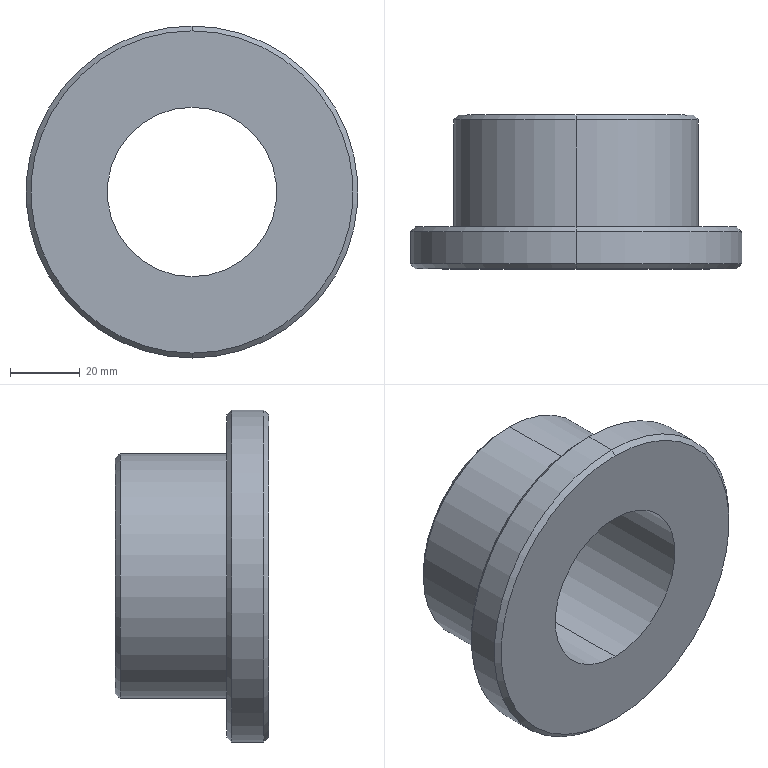Part | SolidWorks | features BaseBody 1 | 1 solid | 15 faces | box 95 x 44 x 95 mm | volume 126129 mm3 | cylinder 6 | cone 6 | plane 3 | commonest cylinder face diameters 48.5 x2 70 x2 95 x2
STEP:
#1=CARTESIAN_POINT('',(0.,0.,-24.25));
#2=VERTEX_POINT('',#1);
#3=CARTESIAN_POINT('',(0.,0.,24.25));
#4=VERTEX_POINT('',#3);
#5=CARTESIAN_POINT('',(0.,0.,0.));
#6=DIRECTION('',(0.,1.,0.));
#7=DIRECTION('',(0.,0.,1.));
#8=AXIS2_PLACEMENT_3D('',#5,#6,#7);
#9=CIRCLE('',#8,24.25);
#10=EDGE_CURVE('',#2,#4,#9,.T.);
#11=ORIENTED_EDGE('',*,*,#10,.F.);
#12=CARTESIAN_POINT('',(0.,44.,-24.25));
#13=VERTEX_POINT('',#12);
#14=CARTESIAN_POINT('',(0.,44.,-24.25));
#15=DIRECTION('',(0.,1.,0.));
#16=VECTOR('',#15,1000.);
#17=LINE('',#14,#16);
#18=EDGE_CURVE('',#2,#13,#17,.T.);
#19=ORIENTED_EDGE('',*,*,#18,.T.);
#20=CARTESIAN_POINT('',(0.,44.,24.25));
#21=VERTEX_POINT('',#20);
#22=CARTESIAN_POINT('',(0.,44.,0.));
#23=DIRECTION('',(0.,1.,0.));
#24=DIRECTION('',(0.,0.,1.));
#25=AXIS2_PLACEMENT_3D('',#22,#23,#24);
#26=CIRCLE('',#25,24.25);
#27=EDGE_CURVE('',#13,#21,#26,.T.);
#28=ORIENTED_EDGE('',*,*,#27,.T.);
#29=CARTESIAN_POINT('',(0.,44.,24.25));
#30=DIRECTION('',(0.,1.,0.));
#31=VECTOR('',#30,1000.);
#32=LINE('',#29,#31);
#33=EDGE_CURVE('',#4,#21,#32,.T.);
#34=ORIENTED_EDGE('',*,*,#33,.F.);
#35=EDGE_LOOP('',(#11,#19,#28,#34));
#36=FACE_OUTER_BOUND('',#35,.T.);
#37=CARTESIAN_POINT('',(0.,44.,0.));
#38=DIRECTION('',(0.,1.,0.));
#39=DIRECTION('',(0.,0.,1.));
#40=AXIS2_PLACEMENT_3D('',#37,#38,#39);
#41=CYLINDRICAL_SURFACE('',#40,24.25);
#42=ADVANCED_FACE('',(#36),#41,.F.);
#43=CARTESIAN_POINT('',(0.,44.,33.6));
#44=VERTEX_POINT('',#43);
#45=CARTESIAN_POINT('',(0.,44.,-33.6));
#46=VERTEX_POINT('',#45);
#47=CARTESIAN_POINT('',(0.,44.,0.));
#48=DIRECTION('',(0.,1.,0.));
#49=DIRECTION('',(0.,0.,1.));
#50=AXIS2_PLACEMENT_3D('',#47,#48,#49);
#51=CIRCLE('',#50,33.6);
#52=EDGE_CURVE('',#44,#46,#51,.T.);
#53=ORIENTED_EDGE('',*,*,#52,.F.);
#54=CARTESIAN_POINT('',(0.,42.6,35.));
#55=VERTEX_POINT('',#54);
#56=CARTESIAN_POINT('',(0.,44.,33.6));
#57=DIRECTION('',(0.,-0.7071,0.7071));
#58=VECTOR('',#57,1000.);
#59=LINE('',#56,#58);
#60=EDGE_CURVE('',#44,#55,#59,.T.);
#61=ORIENTED_EDGE('',*,*,#60,.T.);
#62=CARTESIAN_POINT('',(0.,42.6,-35.));
#63=VERTEX_POINT('',#62);
#64=CARTESIAN_POINT('',(0.,42.6,0.));
#65=DIRECTION('',(0.,-1.,0.));
#66=DIRECTION('',(0.,0.,1.));
#67=AXIS2_PLACEMENT_3D('',#64,#65,#66);
#68=CIRCLE('',#67,35.);
#69=EDGE_CURVE('',#63,#55,#68,.T.);
#70=ORIENTED_EDGE('',*,*,#69,.F.);
#71=CARTESIAN_POINT('',(0.,44.,-33.6));
#72=DIRECTION('',(0.,-0.7071,-0.7071));
#73=VECTOR('',#72,1000.);
#74=LINE('',#71,#73);
#75=EDGE_CURVE('',#46,#63,#74,.T.);
#76=ORIENTED_EDGE('',*,*,#75,.F.);
#77=EDGE_LOOP('',(#53,#61,#70,#76));
#78=FACE_OUTER_BOUND('',#77,.T.);
#79=CARTESIAN_POINT('',(0.,44.,0.));
#80=DIRECTION('',(0.,-1.,0.));
#81=DIRECTION('',(0.,0.,-1.));
#82=AXIS2_PLACEMENT_3D('',#79,#80,#81);
#83=CONICAL_SURFACE('',#82,33.6,0.7854);
#84=ADVANCED_FACE('',(#78),#83,.T.);
#85=ORIENTED_EDGE('',*,*,#69,.T.);
#86=CARTESIAN_POINT('',(0.,12.,35.));
#87=VERTEX_POINT('',#86);
#88=CARTESIAN_POINT('',(0.,44.,35.));
#89=DIRECTION('',(0.,-1.,0.));
#90=VECTOR('',#89,1000.);
#91=LINE('',#88,#90);
#92=EDGE_CURVE('',#55,#87,#91,.T.);
#93=ORIENTED_EDGE('',*,*,#92,.T.);
#94=CARTESIAN_POINT('',(0.,12.,-35.));
#95=VERTEX_POINT('',#94);
#96=CARTESIAN_POINT('',(0.,12.,0.));
#97=DIRECTION('',(0.,1.,0.));
#98=DIRECTION('',(0.,0.,1.));
#99=AXIS2_PLACEMENT_3D('',#96,#97,#98);
#100=CIRCLE('',#99,35.);
#101=EDGE_CURVE('',#87,#95,#100,.T.);
#102=ORIENTED_EDGE('',*,*,#101,.T.);
#103=CARTESIAN_POINT('',(0.,44.,-35.));
#104=DIRECTION('',(0.,-1.,0.));
#105=VECTOR('',#104,1000.);
#106=LINE('',#103,#105);
#107=EDGE_CURVE('',#63,#95,#106,.T.);
#108=ORIENTED_EDGE('',*,*,#107,.F.);
#109=EDGE_LOOP('',(#85,#93,#102,#108));
#110=FACE_OUTER_BOUND('',#109,.T.);
#111=CARTESIAN_POINT('',(0.,44.,0.));
#112=DIRECTION('',(0.,-1.,0.));
#113=DIRECTION('',(0.,0.,-1.));
#114=AXIS2_PLACEMENT_3D('',#111,#112,#113);
#115=CYLINDRICAL_SURFACE('',#114,35.);
#116=ADVANCED_FACE('',(#110),#115,.T.);
#117=CARTESIAN_POINT('',(0.,12.,46.1));
#118=VERTEX_POINT('',#117);
#119=CARTESIAN_POINT('',(0.,12.,-46.1));
#120=VERTEX_POINT('',#119);
#121=CARTESIAN_POINT('',(0.,12.,0.));
#122=DIRECTION('',(0.,1.,0.));
#123=DIRECTION('',(0.,0.,1.));
#124=AXIS2_PLACEMENT_3D('',#121,#122,#123);
#125=CIRCLE('',#124,46.1);
#126=EDGE_CURVE('',#118,#120,#125,.T.);
#127=ORIENTED_EDGE('',*,*,#126,.F.);
#128=CARTESIAN_POINT('',(0.,10.6,47.5));
#129=VERTEX_POINT('',#128);
#130=CARTESIAN_POINT('',(0.,12.,46.1));
#131=DIRECTION('',(0.,-0.7071,0.7071));
#132=VECTOR('',#131,1000.);
#133=LINE('',#130,#132);
#134=EDGE_CURVE('',#118,#129,#133,.T.);
#135=ORIENTED_EDGE('',*,*,#134,.T.);
#136=CARTESIAN_POINT('',(0.,10.6,-47.5));
#137=VERTEX_POINT('',#136);
#138=CARTESIAN_POINT('',(0.,10.6,0.));
#139=DIRECTION('',(0.,-1.,0.));
#140=DIRECTION('',(0.,0.,1.));
#141=AXIS2_PLACEMENT_3D('',#138,#139,#140);
#142=CIRCLE('',#141,47.5);
#143=EDGE_CURVE('',#137,#129,#142,.T.);
#144=ORIENTED_EDGE('',*,*,#143,.F.);
#145=CARTESIAN_POINT('',(0.,12.,-46.1));
#146=DIRECTION('',(0.,-0.7071,-0.7071));
#147=VECTOR('',#146,1000.);
#148=LINE('',#145,#147);
#149=EDGE_CURVE('',#120,#137,#148,.T.);
#150=ORIENTED_EDGE('',*,*,#149,.F.);
#151=EDGE_LOOP('',(#127,#135,#144,#150));
#152=FACE_OUTER_BOUND('',#151,.T.);
#153=CARTESIAN_POINT('',(0.,12.,0.));
#154=DIRECTION('',(0.,-1.,0.));
#155=DIRECTION('',(0.,0.,-1.));
#156=AXIS2_PLACEMENT_3D('',#153,#154,#155);
#157=CONICAL_SURFACE('',#156,46.1,0.7854);
#158=ADVANCED_FACE('',(#152),#157,.T.);
#159=CARTESIAN_POINT('',(0.,0.,-46.1));
#160=VERTEX_POINT('',#159);
#161=CARTESIAN_POINT('',(0.,0.,46.1));
#162=VERTEX_POINT('',#161);
#163=CARTESIAN_POINT('',(0.,0.,0.));
#164=DIRECTION('',(0.,-1.,0.));
#165=DIRECTION('',(0.,0.,1.));
#166=AXIS2_PLACEMENT_3D('',#163,#164,#165);
#167=CIRCLE('',#166,46.1);
#168=EDGE_CURVE('',#160,#162,#167,.T.);
#169=ORIENTED_EDGE('',*,*,#168,.F.);
#170=CARTESIAN_POINT('',(0.,1.4,-47.5));
#171=VERTEX_POINT('',#170);
#172=CARTESIAN_POINT('',(0.,1.4,-47.5));
#173=DIRECTION('',(0.,0.7071,-0.7071));
#174=VECTOR('',#173,1000.);
#175=LINE('',#172,#174);
#176=EDGE_CURVE('',#160,#171,#175,.T.);
#177=ORIENTED_EDGE('',*,*,#176,.T.);
#178=CARTESIAN_POINT('',(0.,1.4,47.5));
#179=VERTEX_POINT('',#178);
#180=CARTESIAN_POINT('',(0.,1.4,0.));
#181=DIRECTION('',(0.,1.,0.));
#182=DIRECTION('',(0.,0.,1.));
#183=AXIS2_PLACEMENT_3D('',#180,#181,#182);
#184=CIRCLE('',#183,47.5);
#185=EDGE_CURVE('',#179,#171,#184,.T.);
#186=ORIENTED_EDGE('',*,*,#185,.F.);
#187=CARTESIAN_POINT('',(0.,1.4,47.5));
#188=DIRECTION('',(0.,0.7071,0.7071));
#189=VECTOR('',#188,1000.);
#190=LINE('',#187,#189);
#191=EDGE_CURVE('',#162,#179,#190,.T.);
#192=ORIENTED_EDGE('',*,*,#191,.F.);
#193=EDGE_LOOP('',(#169,#177,#186,#192));
#194=FACE_OUTER_BOUND('',#193,.T.);
#195=CARTESIAN_POINT('',(0.,1.4,0.));
#196=DIRECTION('',(0.,1.,0.));
#197=DIRECTION('',(0.,0.,1.));
#198=AXIS2_PLACEMENT_3D('',#195,#196,#197);
#199=CONICAL_SURFACE('',#198,47.5,0.7854);
#200=ADVANCED_FACE('',(#194),#199,.T.);
#201=ORIENTED_EDGE('',*,*,#143,.T.);
#202=CARTESIAN_POINT('',(0.,12.,47.5));
#203=DIRECTION('',(0.,-1.,0.));
#204=VECTOR('',#203,1000.);
#205=LINE('',#202,#204);
#206=EDGE_CURVE('',#129,#179,#205,.T.);
#207=ORIENTED_EDGE('',*,*,#206,.T.);
#208=ORIENTED_EDGE('',*,*,#185,.T.);
#209=CARTESIAN_POINT('',(0.,12.,-47.5));
#210=DIRECTION('',(0.,-1.,0.));
#211=VECTOR('',#210,1000.);
#212=LINE('',#209,#211);
#213=EDGE_CURVE('',#137,#171,#212,.T.);
#214=ORIENTED_EDGE('',*,*,#213,.F.);
#215=EDGE_LOOP('',(#201,#207,#208,#214));
#216=FACE_OUTER_BOUND('',#215,.T.);
#217=CARTESIAN_POINT('',(0.,12.,0.));
#218=DIRECTION('',(0.,-1.,0.));
#219=DIRECTION('',(0.,0.,-1.));
#220=AXIS2_PLACEMENT_3D('',#217,#218,#219);
#221=CYLINDRICAL_SURFACE('',#220,47.5);
#222=ADVANCED_FACE('',(#216),#221,.T.);
#223=ORIENTED_EDGE('',*,*,#206,.F.);
#224=CARTESIAN_POINT('',(0.,10.6,0.));
#225=DIRECTION('',(0.,-1.,0.));
#226=DIRECTION('',(0.,0.,1.));
#227=AXIS2_PLACEMENT_3D('',#224,#225,#226);
#228=CIRCLE('',#227,47.5);
#229=EDGE_CURVE('',#129,#137,#228,.T.);
#230=ORIENTED_EDGE('',*,*,#229,.T.);
#231=ORIENTED_EDGE('',*,*,#213,.T.);
#232=CARTESIAN_POINT('',(0.,1.4,0.));
#233=DIRECTION('',(0.,1.,0.));
#234=DIRECTION('',(0.,0.,1.));
#235=AXIS2_PLACEMENT_3D('',#232,#233,#234);
#236=CIRCLE('',#235,47.5);
#237=EDGE_CURVE('',#171,#179,#236,.T.);
#238=ORIENTED_EDGE('',*,*,#237,.T.);
#239=EDGE_LOOP('',(#223,#230,#231,#238));
#240=FACE_OUTER_BOUND('',#239,.T.);
#241=CARTESIAN_POINT('',(0.,12.,0.));
#242=DIRECTION('',(0.,-1.,0.));
#243=DIRECTION('',(0.,0.,-1.));
#244=AXIS2_PLACEMENT_3D('',#241,#242,#243);
#245=CYLINDRICAL_SURFACE('',#244,47.5);
#246=ADVANCED_FACE('',(#240),#245,.T.);
#247=CARTESIAN_POINT('',(0.,12.,0.));
#248=DIRECTION('',(0.,1.,0.));
#249=DIRECTION('',(0.,0.,1.));
#250=AXIS2_PLACEMENT_3D('',#247,#248,#249);
#251=CIRCLE('',#250,35.);
#252=EDGE_CURVE('',#95,#87,#251,.T.);
#253=ORIENTED_EDGE('',*,*,#252,.F.);
#254=ORIENTED_EDGE('',*,*,#101,.F.);
#255=EDGE_LOOP('',(#253,#254));
#256=FACE_BOUND('',#255,.T.);
#257=CARTESIAN_POINT('',(0.,12.,0.));
#258=DIRECTION('',(0.,1.,0.));
#259=DIRECTION('',(0.,0.,1.));
#260=AXIS2_PLACEMENT_3D('',#257,#258,#259);
#261=CIRCLE('',#260,46.1);
#262=EDGE_CURVE('',#120,#118,#261,.T.);
#263=ORIENTED_EDGE('',*,*,#262,.T.);
#264=ORIENTED_EDGE('',*,*,#126,.T.);
#265=EDGE_LOOP('',(#263,#264));
#266=FACE_OUTER_BOUND('',#265,.T.);
#267=CARTESIAN_POINT('',(0.,12.,0.));
#268=DIRECTION('',(0.,1.,0.));
#269=DIRECTION('',(0.,0.,1.));
#270=AXIS2_PLACEMENT_3D('',#267,#268,#269);
#271=PLANE('',#270);
#272=ADVANCED_FACE('',(#256,#266),#271,.T.);
#273=CARTESIAN_POINT('',(0.,0.,0.));
#274=DIRECTION('',(0.,1.,0.));
#275=DIRECTION('',(0.,0.,1.));
#276=AXIS2_PLACEMENT_3D('',#273,#274,#275);
#277=CIRCLE('',#276,24.25);
#278=EDGE_CURVE('',#4,#2,#277,.T.);
#279=ORIENTED_EDGE('',*,*,#278,.T.);
#280=ORIENTED_EDGE('',*,*,#10,.T.);
#281=EDGE_LOOP('',(#279,#280));
#282=FACE_BOUND('',#281,.T.);
#283=CARTESIAN_POINT('',(0.,0.,0.));
#284=DIRECTION('',(0.,-1.,0.));
#285=DIRECTION('',(0.,0.,1.));
#286=AXIS2_PLACEMENT_3D('',#283,#284,#285);
#287=CIRCLE('',#286,46.1);
#288=EDGE_CURVE('',#162,#160,#287,.T.);
#289=ORIENTED_EDGE('',*,*,#288,.T.);
#290=ORIENTED_EDGE('',*,*,#168,.T.);
#291=EDGE_LOOP('',(#289,#290));
#292=FACE_OUTER_BOUND('',#291,.T.);
#293=CARTESIAN_POINT('',(0.,0.,0.));
#294=DIRECTION('',(0.,1.,0.));
#295=DIRECTION('',(0.,0.,1.));
#296=AXIS2_PLACEMENT_3D('',#293,#294,#295);
#297=PLANE('',#296);
#298=ADVANCED_FACE('',(#282,#292),#297,.F.);
#299=ORIENTED_EDGE('',*,*,#176,.F.);
#300=ORIENTED_EDGE('',*,*,#288,.F.);
#301=ORIENTED_EDGE('',*,*,#191,.T.);
#302=ORIENTED_EDGE('',*,*,#237,.F.);
#303=EDGE_LOOP('',(#299,#300,#301,#302));
#304=FACE_OUTER_BOUND('',#303,.T.);
#305=CARTESIAN_POINT('',(0.,1.4,0.));
#306=DIRECTION('',(0.,1.,0.));
#307=DIRECTION('',(0.,0.,1.));
#308=AXIS2_PLACEMENT_3D('',#305,#306,#307);
#309=CONICAL_SURFACE('',#308,47.5,0.7854);
#310=ADVANCED_FACE('',(#304),#309,.T.);
#311=ORIENTED_EDGE('',*,*,#134,.F.);
#312=ORIENTED_EDGE('',*,*,#262,.F.);
#313=ORIENTED_EDGE('',*,*,#149,.T.);
#314=ORIENTED_EDGE('',*,*,#229,.F.);
#315=EDGE_LOOP('',(#311,#312,#313,#314));
#316=FACE_OUTER_BOUND('',#315,.T.);
#317=CARTESIAN_POINT('',(0.,12.,0.));
#318=DIRECTION('',(0.,-1.,0.));
#319=DIRECTION('',(0.,0.,-1.));
#320=AXIS2_PLACEMENT_3D('',#317,#318,#319);
#321=CONICAL_SURFACE('',#320,46.1,0.7854);
#322=ADVANCED_FACE('',(#316),#321,.T.);
#323=ORIENTED_EDGE('',*,*,#92,.F.);
#324=CARTESIAN_POINT('',(0.,42.6,0.));
#325=DIRECTION('',(0.,-1.,0.));
#326=DIRECTION('',(0.,0.,1.));
#327=AXIS2_PLACEMENT_3D('',#324,#325,#326);
#328=CIRCLE('',#327,35.);
#329=EDGE_CURVE('',#55,#63,#328,.T.);
#330=ORIENTED_EDGE('',*,*,#329,.T.);
#331=ORIENTED_EDGE('',*,*,#107,.T.);
#332=ORIENTED_EDGE('',*,*,#252,.T.);
#333=EDGE_LOOP('',(#323,#330,#331,#332));
#334=FACE_OUTER_BOUND('',#333,.T.);
#335=CARTESIAN_POINT('',(0.,44.,0.));
#336=DIRECTION('',(0.,-1.,0.));
#337=DIRECTION('',(0.,0.,-1.));
#338=AXIS2_PLACEMENT_3D('',#335,#336,#337);
#339=CYLINDRICAL_SURFACE('',#338,35.);
#340=ADVANCED_FACE('',(#334),#339,.T.);
#341=CARTESIAN_POINT('',(0.,44.,0.));
#342=DIRECTION('',(0.,1.,0.));
#343=DIRECTION('',(0.,0.,1.));
#344=AXIS2_PLACEMENT_3D('',#341,#342,#343);
#345=CIRCLE('',#344,24.25);
#346=EDGE_CURVE('',#21,#13,#345,.T.);
#347=ORIENTED_EDGE('',*,*,#346,.F.);
#348=ORIENTED_EDGE('',*,*,#27,.F.);
#349=EDGE_LOOP('',(#347,#348));
#350=FACE_BOUND('',#349,.T.);
#351=CARTESIAN_POINT('',(0.,44.,0.));
#352=DIRECTION('',(0.,1.,0.));
#353=DIRECTION('',(0.,0.,1.));
#354=AXIS2_PLACEMENT_3D('',#351,#352,#353);
#355=CIRCLE('',#354,33.6);
#356=EDGE_CURVE('',#46,#44,#355,.T.);
#357=ORIENTED_EDGE('',*,*,#356,.T.);
#358=ORIENTED_EDGE('',*,*,#52,.T.);
#359=EDGE_LOOP('',(#357,#358));
#360=FACE_OUTER_BOUND('',#359,.T.);
#361=CARTESIAN_POINT('',(0.,44.,0.));
#362=DIRECTION('',(0.,1.,0.));
#363=DIRECTION('',(0.,0.,1.));
#364=AXIS2_PLACEMENT_3D('',#361,#362,#363);
#365=PLANE('',#364);
#366=ADVANCED_FACE('',(#350,#360),#365,.T.);
#367=ORIENTED_EDGE('',*,*,#60,.F.);
#368=ORIENTED_EDGE('',*,*,#356,.F.);
#369=ORIENTED_EDGE('',*,*,#75,.T.);
#370=ORIENTED_EDGE('',*,*,#329,.F.);
#371=EDGE_LOOP('',(#367,#368,#369,#370));
#372=FACE_OUTER_BOUND('',#371,.T.);
#373=CARTESIAN_POINT('',(0.,44.,0.));
#374=DIRECTION('',(0.,-1.,0.));
#375=DIRECTION('',(0.,0.,-1.));
#376=AXIS2_PLACEMENT_3D('',#373,#374,#375);
#377=CONICAL_SURFACE('',#376,33.6,0.7854);
#378=ADVANCED_FACE('',(#372),#377,.T.);
#379=ORIENTED_EDGE('',*,*,#18,.F.);
#380=ORIENTED_EDGE('',*,*,#278,.F.);
#381=ORIENTED_EDGE('',*,*,#33,.T.);
#382=ORIENTED_EDGE('',*,*,#346,.T.);
#383=EDGE_LOOP('',(#379,#380,#381,#382));
#384=FACE_OUTER_BOUND('',#383,.T.);
#385=CARTESIAN_POINT('',(0.,44.,0.));
#386=DIRECTION('',(0.,1.,0.));
#387=DIRECTION('',(0.,0.,1.));
#388=AXIS2_PLACEMENT_3D('',#385,#386,#387);
#389=CYLINDRICAL_SURFACE('',#388,24.25);
#390=ADVANCED_FACE('',(#384),#389,.F.);
#391=CLOSED_SHELL('',(#42,#84,#116,#158,#200,#222,#246,#272,#298,#310,#322,#340,#366,#378,#390));
#392=MANIFOLD_SOLID_BREP('',#391);
#393=CARTESIAN_POINT('',(0.,0.,0.));
#394=DIRECTION('',(0.,0.,1.));
#395=DIRECTION('',(1.,0.,0.));
#396=AXIS2_PLACEMENT_3D('',#393,#394,#395);
#397=(LENGTH_UNIT()NAMED_UNIT(*)SI_UNIT(.MILLI.,.METRE.));
#398=UNCERTAINTY_MEASURE_WITH_UNIT(LENGTH_MEASURE(0.00001),#397,'','');
#399=(NAMED_UNIT(*)PLANE_ANGLE_UNIT()SI_UNIT($,.RADIAN.));
#400=(NAMED_UNIT(*)SI_UNIT($,.STERADIAN.)SOLID_ANGLE_UNIT());
#401=(GEOMETRIC_REPRESENTATION_CONTEXT(3)GLOBAL_UNCERTAINTY_ASSIGNED_CONTEXT((#398))GLOBAL_UNIT_ASSIGNED_CONTEXT((#397,#399,#400))REPRESENTATION_CONTEXT('',''));
#402=ADVANCED_BREP_SHAPE_REPRESENTATION('',(#392,#396),#401);